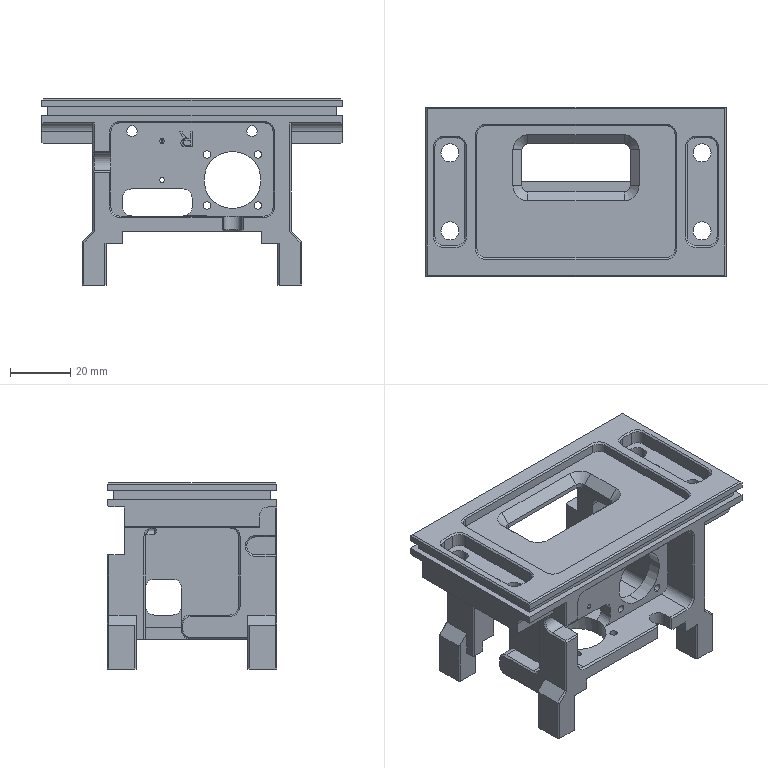NC program | Mastercam | posted with a generic post | part box 100 x 56.5 x 62 mm
Lines 28426 to 30392 of 45570, first 1501 of 1967 lines:
N6980 T16 M6
N6990 G0 G90 G17 G54 X59.6 Y2.263 A0. S5500 M3
N7000 G43 H16 Z20. M8
N7010 Z1.
N7020 G1 Z-28.5 F600.
N7030 X58.469 Y1.131 F1000.
N7040 G3 X58. Y0. I1.131 J-1.131
N7050 G1 Y-31.
N7060 G2 X50. Y-39. I-8. J0.
N7070 G1 X-50.
N7080 G2 X-58. Y-31. I0. J8.
N7090 G1 Y31.
N7100 G2 X-50. Y39. I8. J0.
N7110 G1 X50.
N7120 G2 X58. Y31. I0. J-8.
N7130 G1 Y0.
N7140 Y-.5
N7150 G3 X58.469 Y-1.631 I1.6 J0.
N7160 G1 X59.6 Y-2.763
N7170 Y2.263
N7180 Z-57. F600.
N7190 X58.469 Y1.131 F1000.
N7200 G3 X58. Y0. I1.131 J-1.131
N7210 G1 Y-31.
N7220 G2 X50. Y-39. I-8. J0.
N7230 G1 X-50.
N7240 G2 X-58. Y-31. I0. J8.
N7250 G1 Y31.
N7260 G2 X-50. Y39. I8. J0.
N7270 G1 X50.
N7280 G2 X58. Y31. I0. J-8.
N7290 G1 Y0.
N7300 Y-.5
N7310 G3 X58.469 Y-1.631 I1.6 J0.
N7320 G1 X59.6 Y-2.763
N7330 G0 Z20.
N7340 M5
N7350 G91 G28 Z0. M9
N7360 A0.
N7370 M01
N7380 T6 M6
N7390 G0 G90 G17 G54 X16.314 Y-19.3 A0. S7000 M3
N7400 G43 H6 Z20. M8
N7410 Z1.
N7420 G1 Z-.496 F600.
N7430 X16.738 Y-19.724 F3000.
N7440 G3 X17.162 Y-19.9 I.424 J.424
N7450 G1 X23.9
N7460 Y-13.87
N7470 G3 X23.724 Y-13.445 I-.6 J0.
N7480 G1 X23.3 Y-13.021
N7490 X16.314 Y-19.3
N7500 Z-.992 F600.
N7510 X16.738 Y-19.724 F3000.
N7520 G3 X17.162 Y-19.9 I.424 J.424
N7530 G1 X23.9
N7540 Y-13.87
N7550 G3 X23.724 Y-13.445 I-.6 J0.
N7560 G1 X23.3 Y-13.021
N7570 X16.314 Y-19.3
N7580 Z-1.488 F600.
N7590 X16.738 Y-19.724 F3000.
N7600 G3 X17.162 Y-19.9 I.424 J.424
N7610 G1 X23.9
N7620 Y-13.87
N7630 G3 X23.724 Y-13.445 I-.6 J0.
N7640 G1 X23.3 Y-13.021
N7650 X16.314 Y-19.3
N7660 Z-1.983 F600.
N7670 X16.738 Y-19.724 F3000.
N7680 G3 X17.162 Y-19.9 I.424 J.424
N7690 G1 X23.9
N7700 Y-13.87
N7710 G3 X23.724 Y-13.445 I-.6 J0.
N7720 G1 X23.3 Y-13.021
N7730 X16.314 Y-19.3
N7740 Z-2.479 F600.
N7750 X16.738 Y-19.724 F3000.
N7760 G3 X17.162 Y-19.9 I.424 J.424
N7770 G1 X23.9
N7780 Y-13.87
N7790 G3 X23.724 Y-13.445 I-.6 J0.
N7800 G1 X23.3 Y-13.021
N7810 X16.314 Y-19.3
N7820 Z-2.975 F600.
N7830 X16.738 Y-19.724 F3000.
N7840 G3 X17.162 Y-19.9 I.424 J.424
N7850 G1 X23.9
N7860 Y-13.87
N7870 G3 X23.724 Y-13.445 I-.6 J0.
N7880 G1 X23.3 Y-13.021
N7890 X16.314 Y-19.3
N7900 Z-3.471 F600.
N7910 X16.738 Y-19.724 F3000.
N7920 G3 X17.162 Y-19.9 I.424 J.424
N7930 G1 X23.9
N7940 Y-13.87
N7950 G3 X23.724 Y-13.445 I-.6 J0.
N7960 G1 X23.3 Y-13.021
N7970 X16.314 Y-19.3
N7980 Z-3.967 F600.
N7990 X16.738 Y-19.724 F3000.
N8000 G3 X17.162 Y-19.9 I.424 J.424
N8010 G1 X23.9
N8020 Y-13.87
N8030 G3 X23.724 Y-13.445 I-.6 J0.
N8040 G1 X23.3 Y-13.021
N8050 X16.314 Y-19.3
N8060 Z-4.463 F600.
N8070 X16.738 Y-19.724 F3000.
N8080 G3 X17.162 Y-19.9 I.424 J.424
N8090 G1 X23.9
N8100 Y-13.87
N8110 G3 X23.724 Y-13.445 I-.6 J0.
N8120 G1 X23.3 Y-13.021
N8130 X16.314 Y-19.3
N8140 Z-4.958 F600.
N8150 X16.738 Y-19.724 F3000.
N8160 G3 X17.162 Y-19.9 I.424 J.424
N8170 G1 X23.9
N8180 Y-13.87
N8190 G3 X23.724 Y-13.445 I-.6 J0.
N8200 G1 X23.3 Y-13.021
N8210 X16.314 Y-19.3
N8220 Z-5.454 F600.
N8230 X16.738 Y-19.724 F3000.
N8240 G3 X17.162 Y-19.9 I.424 J.424
N8250 G1 X23.9
N8260 Y-13.87
N8270 G3 X23.724 Y-13.445 I-.6 J0.
N8280 G1 X23.3 Y-13.021
N8290 X16.314 Y-19.3
N8300 Z-5.95 F600.
N8310 X16.738 Y-19.724 F3000.
N8320 G3 X17.162 Y-19.9 I.424 J.424
N8330 G1 X23.9
N8340 Y-13.87
N8350 G3 X23.724 Y-13.445 I-.6 J0.
N8360 G1 X23.3 Y-13.021
N8370 X16.314 Y-19.3
N8380 Z-6.446 F600.
N8390 X16.738 Y-19.724 F3000.
N8400 G3 X17.162 Y-19.9 I.424 J.424
N8410 G1 X23.9
N8420 Y-13.87
N8430 G3 X23.724 Y-13.445 I-.6 J0.
N8440 G1 X23.3 Y-13.021
N8450 X16.314 Y-19.3
N8460 Z-6.942 F600.
N8470 X16.738 Y-19.724 F3000.
N8480 G3 X17.162 Y-19.9 I.424 J.424
N8490 G1 X23.9
N8500 Y-13.87
N8510 G3 X23.724 Y-13.445 I-.6 J0.
N8520 G1 X23.3 Y-13.021
N8530 X16.314 Y-19.3
N8540 Z-7.438 F600.
N8550 X16.738 Y-19.724 F3000.
N8560 G3 X17.162 Y-19.9 I.424 J.424
N8570 G1 X23.9
N8580 Y-13.87
N8590 G3 X23.724 Y-13.445 I-.6 J0.
N8600 G1 X23.3 Y-13.021
N8610 X16.314 Y-19.3
N8620 Z-7.933 F600.
N8630 X16.738 Y-19.724 F3000.
N8640 G3 X17.162 Y-19.9 I.424 J.424
N8650 G1 X23.9
N8660 Y-13.87
N8670 G3 X23.724 Y-13.445 I-.6 J0.
N8680 G1 X23.3 Y-13.021
N8690 X16.314 Y-19.3
N8700 Z-8.429 F600.
N8710 X16.738 Y-19.724 F3000.
N8720 G3 X17.162 Y-19.9 I.424 J.424
N8730 G1 X23.9
N8740 Y-13.87
N8750 G3 X23.724 Y-13.445 I-.6 J0.
N8760 G1 X23.3 Y-13.021
N8770 X16.314 Y-19.3
N8780 Z-8.925 F600.
N8790 X16.738 Y-19.724 F3000.
N8800 G3 X17.162 Y-19.9 I.424 J.424
N8810 G1 X23.9
N8820 Y-13.87
N8830 G3 X23.724 Y-13.445 I-.6 J0.
N8840 G1 X23.3 Y-13.021
N8850 X16.314 Y-19.3
N8860 Z-9.421 F600.
N8870 X16.738 Y-19.724 F3000.
N8880 G3 X17.162 Y-19.9 I.424 J.424
N8890 G1 X23.9
N8900 Y-13.87
N8910 G3 X23.724 Y-13.445 I-.6 J0.
N8920 G1 X23.3 Y-13.021
N8930 X16.314 Y-19.3
N8940 Z-9.917 F600.
N8950 X16.738 Y-19.724 F3000.
N8960 G3 X17.162 Y-19.9 I.424 J.424
N8970 G1 X23.9
N8980 Y-13.87
N8990 G3 X23.724 Y-13.445 I-.6 J0.
N9000 G1 X23.3 Y-13.021
N9010 X16.314 Y-19.3
N9020 Z-10.412 F600.
N9030 X16.738 Y-19.724 F3000.
N9040 G3 X17.162 Y-19.9 I.424 J.424
N9050 G1 X23.9
N9060 Y-13.87
N9070 G3 X23.724 Y-13.445 I-.6 J0.
N9080 G1 X23.3 Y-13.021
N9090 X16.314 Y-19.3
N9100 Z-10.908 F600.
N9110 X16.738 Y-19.724 F3000.
N9120 G3 X17.162 Y-19.9 I.424 J.424
N9130 G1 X23.9
N9140 Y-13.87
N9150 G3 X23.724 Y-13.445 I-.6 J0.
N9160 G1 X23.3 Y-13.021
N9170 X16.314 Y-19.3
N9180 Z-11.404 F600.
N9190 X16.738 Y-19.724 F3000.
N9200 G3 X17.162 Y-19.9 I.424 J.424
N9210 G1 X23.9
N9220 Y-13.87
N9230 G3 X23.724 Y-13.445 I-.6 J0.
N9240 G1 X23.3 Y-13.021
N9250 X16.314 Y-19.3
N9260 Z-11.9 F600.
N9270 X16.738 Y-19.724 F3000.
N9280 G3 X17.162 Y-19.9 I.424 J.424
N9290 G1 X23.9
N9300 Y-13.87
N9310 G3 X23.724 Y-13.445 I-.6 J0.
N9320 G1 X23.3 Y-13.021
N9330 G0 Z20.
N9340 X-23.3
N9350 Z1.
N9360 G1 Z-.496 F600.
N9370 X-23.724 Y-13.445 F3000.
N9380 G3 X-23.9 Y-13.869 I.424 J-.424
N9390 G1 Y-19.9
N9400 X-17.162
N9410 G3 X-16.738 Y-19.724 I0. J.6
N9420 G1 X-16.314 Y-19.3
N9430 X-23.3 Y-13.021
N9440 Z-.992 F600.
N9450 X-23.724 Y-13.445 F3000.
N9460 G3 X-23.9 Y-13.869 I.424 J-.424
N9470 G1 Y-19.9
N9480 X-17.162
N9490 G3 X-16.738 Y-19.724 I0. J.6
N9500 G1 X-16.314 Y-19.3
N9510 X-23.3 Y-13.021
N9520 Z-1.488 F600.
N9530 X-23.724 Y-13.445 F3000.
N9540 G3 X-23.9 Y-13.869 I.424 J-.424
N9550 G1 Y-19.9
N9560 X-17.162
N9570 G3 X-16.738 Y-19.724 I0. J.6
N9580 G1 X-16.314 Y-19.3
N9590 X-23.3 Y-13.021
N9600 Z-1.983 F600.
N9610 X-23.724 Y-13.445 F3000.
N9620 G3 X-23.9 Y-13.869 I.424 J-.424
N9630 G1 Y-19.9
N9640 X-17.162
N9650 G3 X-16.738 Y-19.724 I0. J.6
N9660 G1 X-16.314 Y-19.3
N9670 X-23.3 Y-13.021
N9680 Z-2.479 F600.
N9690 X-23.724 Y-13.445 F3000.
N9700 G3 X-23.9 Y-13.869 I.424 J-.424
N9710 G1 Y-19.9
N9720 X-17.162
N9730 G3 X-16.738 Y-19.724 I0. J.6
N9740 G1 X-16.314 Y-19.3
N9750 X-23.3 Y-13.021
N9760 Z-2.975 F600.
N9770 X-23.724 Y-13.445 F3000.
N9780 G3 X-23.9 Y-13.869 I.424 J-.424
N9790 G1 Y-19.9
N9800 X-17.162
N9810 G3 X-16.738 Y-19.724 I0. J.6
N9820 G1 X-16.314 Y-19.3
N9830 X-23.3 Y-13.021
N9840 Z-3.471 F600.
N9850 X-23.724 Y-13.445 F3000.
N9860 G3 X-23.9 Y-13.869 I.424 J-.424
N9870 G1 Y-19.9
N9880 X-17.162
N9890 G3 X-16.738 Y-19.724 I0. J.6
N9900 G1 X-16.314 Y-19.3
N9910 X-23.3 Y-13.021
N9920 Z-3.967 F600.
N9930 X-23.724 Y-13.445 F3000.
N9940 G3 X-23.9 Y-13.869 I.424 J-.424
N9950 G1 Y-19.9
N9960 X-17.162
N9970 G3 X-16.738 Y-19.724 I0. J.6
N9980 G1 X-16.314 Y-19.3
N9990 X-23.3 Y-13.021
N100 Z-4.463 F600.
N110 X-23.724 Y-13.445 F3000.
N120 G3 X-23.9 Y-13.869 I.424 J-.424
N130 G1 Y-19.9
N140 X-17.162
N150 G3 X-16.738 Y-19.724 I0. J.6
N160 G1 X-16.314 Y-19.3
N170 X-23.3 Y-13.021
N180 Z-4.958 F600.
N190 X-23.724 Y-13.445 F3000.
N200 G3 X-23.9 Y-13.869 I.424 J-.424
N210 G1 Y-19.9
N220 X-17.162
N230 G3 X-16.738 Y-19.724 I0. J.6
N240 G1 X-16.314 Y-19.3
N250 X-23.3 Y-13.021
N260 Z-5.454 F600.
N270 X-23.724 Y-13.445 F3000.
N280 G3 X-23.9 Y-13.869 I.424 J-.424
N290 G1 Y-19.9
N300 X-17.162
N310 G3 X-16.738 Y-19.724 I0. J.6
N320 G1 X-16.314 Y-19.3
N330 X-23.3 Y-13.021
N340 Z-5.95 F600.
N350 X-23.724 Y-13.445 F3000.
N360 G3 X-23.9 Y-13.869 I.424 J-.424
N370 G1 Y-19.9
N380 X-17.162
N390 G3 X-16.738 Y-19.724 I0. J.6
N400 G1 X-16.314 Y-19.3
N410 X-23.3 Y-13.021
N420 Z-6.446 F600.
N430 X-23.724 Y-13.445 F3000.
N440 G3 X-23.9 Y-13.869 I.424 J-.424
N450 G1 Y-19.9
N460 X-17.162
N470 G3 X-16.738 Y-19.724 I0. J.6
N480 G1 X-16.314 Y-19.3
N490 X-23.3 Y-13.021
N500 Z-6.942 F600.
N510 X-23.724 Y-13.445 F3000.
N520 G3 X-23.9 Y-13.869 I.424 J-.424
N530 G1 Y-19.9
N540 X-17.162
N550 G3 X-16.738 Y-19.724 I0. J.6
N560 G1 X-16.314 Y-19.3
N570 X-23.3 Y-13.021
N580 Z-7.438 F600.
N590 X-23.724 Y-13.445 F3000.
N600 G3 X-23.9 Y-13.869 I.424 J-.424
N610 G1 Y-19.9
N620 X-17.162
N630 G3 X-16.738 Y-19.724 I0. J.6
N640 G1 X-16.314 Y-19.3
N650 X-23.3 Y-13.021
N660 Z-7.933 F600.
N670 X-23.724 Y-13.445 F3000.
N680 G3 X-23.9 Y-13.869 I.424 J-.424
N690 G1 Y-19.9
N700 X-17.162
N710 G3 X-16.738 Y-19.724 I0. J.6
N720 G1 X-16.314 Y-19.3
N730 X-23.3 Y-13.021
N740 Z-8.429 F600.
N750 X-23.724 Y-13.445 F3000.
N760 G3 X-23.9 Y-13.869 I.424 J-.424
N770 G1 Y-19.9
N780 X-17.162
N790 G3 X-16.738 Y-19.724 I0. J.6
N800 G1 X-16.314 Y-19.3
N810 X-23.3 Y-13.021
N820 Z-8.925 F600.
N830 X-23.724 Y-13.445 F3000.
N840 G3 X-23.9 Y-13.869 I.424 J-.424
N850 G1 Y-19.9
N860 X-17.162
N870 G3 X-16.738 Y-19.724 I0. J.6
N880 G1 X-16.314 Y-19.3
N890 X-23.3 Y-13.021
N900 Z-9.421 F600.
N910 X-23.724 Y-13.445 F3000.
N920 G3 X-23.9 Y-13.869 I.424 J-.424
N930 G1 Y-19.9
N940 X-17.162
N950 G3 X-16.738 Y-19.724 I0. J.6
N960 G1 X-16.314 Y-19.3
N970 X-23.3 Y-13.021
N980 Z-9.917 F600.
N990 X-23.724 Y-13.445 F3000.
N1000 G3 X-23.9 Y-13.869 I.424 J-.424
N1010 G1 Y-19.9
N1020 X-17.162
N1030 G3 X-16.738 Y-19.724 I0. J.6
N1040 G1 X-16.314 Y-19.3
N1050 X-23.3 Y-13.021
N1060 Z-10.412 F600.
N1070 X-23.724 Y-13.445 F3000.
N1080 G3 X-23.9 Y-13.869 I.424 J-.424
N1090 G1 Y-19.9
N1100 X-17.162
N1110 G3 X-16.738 Y-19.724 I0. J.6
N1120 G1 X-16.314 Y-19.3
N1130 X-23.3 Y-13.021
N1140 Z-10.908 F600.
N1150 X-23.724 Y-13.445 F3000.
N1160 G3 X-23.9 Y-13.869 I.424 J-.424
N1170 G1 Y-19.9
N1180 X-17.162
N1190 G3 X-16.738 Y-19.724 I0. J.6
N1200 G1 X-16.314 Y-19.3
N1210 X-23.3 Y-13.021
N1220 Z-11.404 F600.
N1230 X-23.724 Y-13.445 F3000.
N1240 G3 X-23.9 Y-13.869 I.424 J-.424
N1250 G1 Y-19.9
N1260 X-17.162
N1270 G3 X-16.738 Y-19.724 I0. J.6
N1280 G1 X-16.314 Y-19.3
N1290 X-23.3 Y-13.021
N1300 Z-11.9 F600.
N1310 X-23.724 Y-13.445 F3000.
N1320 G3 X-23.9 Y-13.869 I.424 J-.424
N1330 G1 Y-19.9
N1340 X-17.162
N1350 G3 X-16.738 Y-19.724 I0. J.6
N1360 G1 X-16.314 Y-19.3
N1370 G0 Z20.
N1380 X-16.603 Y4.3
N1390 Z1.
N1400 G1 Z-.496 F600.
N1410 X-17.027 Y4.724 F3000.
N1420 G3 X-17.451 Y4.9 I-.424 J-.424
N1430 G1 X-23.9
N1440 Y-1.142
N1450 G3 X-23.724 Y-1.567 I.6 J0.
N1460 G1 X-23.3 Y-1.991
N1470 X-16.603 Y4.3
N1480 Z-.992 F600.
N1490 X-17.027 Y4.724 F3000.
N1500 G3 X-17.451 Y4.9 I-.424 J-.424
N1510 G1 X-23.9
N1520 Y-1.142
N1530 G3 X-23.724 Y-1.567 I.6 J0.
N1540 G1 X-23.3 Y-1.991
N1550 X-16.603 Y4.3
N1560 Z-1.488 F600.
N1570 X-17.027 Y4.724 F3000.
N1580 G3 X-17.451 Y4.9 I-.424 J-.424
N1590 G1 X-23.9
N1600 Y-1.142
N1610 G3 X-23.724 Y-1.567 I.6 J0.
N1620 G1 X-23.3 Y-1.991
N1630 X-16.603 Y4.3
N1640 Z-1.983 F600.
N1650 X-17.027 Y4.724 F3000.
N1660 G3 X-17.451 Y4.9 I-.424 J-.424
N1670 G1 X-23.9
N1680 Y-1.142
N1690 G3 X-23.724 Y-1.567 I.6 J0.
N1700 G1 X-23.3 Y-1.991
N1710 X-16.603 Y4.3
N1720 Z-2.479 F600.
N1730 X-17.027 Y4.724 F3000.
N1740 G3 X-17.451 Y4.9 I-.424 J-.424
N1750 G1 X-23.9
N1760 Y-1.142
N1770 G3 X-23.724 Y-1.567 I.6 J0.
N1780 G1 X-23.3 Y-1.991
N1790 X-16.603 Y4.3
N1800 Z-2.975 F600.
N1810 X-17.027 Y4.724 F3000.
N1820 G3 X-17.451 Y4.9 I-.424 J-.424
N1830 G1 X-23.9
N1840 Y-1.142
N1850 G3 X-23.724 Y-1.567 I.6 J0.
N1860 G1 X-23.3 Y-1.991
N1870 X-16.603 Y4.3
N1880 Z-3.471 F600.
N1890 X-17.027 Y4.724 F3000.
N1900 G3 X-17.451 Y4.9 I-.424 J-.424
N1910 G1 X-23.9
N1920 Y-1.142
N1930 G3 X-23.724 Y-1.567 I.6 J0.
N1940 G1 X-23.3 Y-1.991
N1950 X-16.603 Y4.3
N1960 Z-3.967 F600.
N1970 X-17.027 Y4.724 F3000.
N1980 G3 X-17.451 Y4.9 I-.424 J-.424
N1990 G1 X-23.9
N2000 Y-1.142
N2010 G3 X-23.724 Y-1.567 I.6 J0.
N2020 G1 X-23.3 Y-1.991
N2030 X-16.603 Y4.3
N2040 Z-4.463 F600.
N2050 X-17.027 Y4.724 F3000.
N2060 G3 X-17.451 Y4.9 I-.424 J-.424
N2070 G1 X-23.9
N2080 Y-1.142
N2090 G3 X-23.724 Y-1.567 I.6 J0.
N2100 G1 X-23.3 Y-1.991
N2110 X-16.603 Y4.3
N2120 Z-4.958 F600.
N2130 X-17.027 Y4.724 F3000.
N2140 G3 X-17.451 Y4.9 I-.424 J-.424
N2150 G1 X-23.9
N2160 Y-1.142
N2170 G3 X-23.724 Y-1.567 I.6 J0.
N2180 G1 X-23.3 Y-1.991
N2190 X-16.603 Y4.3
N2200 Z-5.454 F600.
N2210 X-17.027 Y4.724 F3000.
N2220 G3 X-17.451 Y4.9 I-.424 J-.424
N2230 G1 X-23.9
N2240 Y-1.142
N2250 G3 X-23.724 Y-1.567 I.6 J0.
N2260 G1 X-23.3 Y-1.991
N2270 X-16.603 Y4.3
N2280 Z-5.95 F600.
N2290 X-17.027 Y4.724 F3000.
N2300 G3 X-17.451 Y4.9 I-.424 J-.424
N2310 G1 X-23.9
N2320 Y-1.142
N2330 G3 X-23.724 Y-1.567 I.6 J0.
N2340 G1 X-23.3 Y-1.991
N2350 X-16.603 Y4.3
N2360 Z-6.446 F600.
N2370 X-17.027 Y4.724 F3000.
N2380 G3 X-17.451 Y4.9 I-.424 J-.424
N2390 G1 X-23.9
N2400 Y-1.142
N2410 G3 X-23.724 Y-1.567 I.6 J0.
N2420 G1 X-23.3 Y-1.991
N2430 X-16.603 Y4.3
N2440 Z-6.942 F600.
N2450 X-17.027 Y4.724 F3000.
N2460 G3 X-17.451 Y4.9 I-.424 J-.424
N2470 G1 X-23.9
N2480 Y-1.142
N2490 G3 X-23.724 Y-1.567 I.6 J0.
N2500 G1 X-23.3 Y-1.991
N2510 X-16.603 Y4.3
N2520 Z-7.438 F600.
N2530 X-17.027 Y4.724 F3000.
N2540 G3 X-17.451 Y4.9 I-.424 J-.424
N2550 G1 X-23.9
N2560 Y-1.142
N2570 G3 X-23.724 Y-1.567 I.6 J0.
N2580 G1 X-23.3 Y-1.991
N2590 X-16.603 Y4.3
N2600 Z-7.933 F600.
N2610 X-17.027 Y4.724 F3000.
N2620 G3 X-17.451 Y4.9 I-.424 J-.424
N2630 G1 X-23.9
N2640 Y-1.142
N2650 G3 X-23.724 Y-1.567 I.6 J0.
N2660 G1 X-23.3 Y-1.991
N2670 X-16.603 Y4.3
N2680 Z-8.429 F600.
N2690 X-17.027 Y4.724 F3000.
N2700 G3 X-17.451 Y4.9 I-.424 J-.424
N2710 G1 X-23.9
N2720 Y-1.142
N2730 G3 X-23.724 Y-1.567 I.6 J0.
N2740 G1 X-23.3 Y-1.991
N2750 X-16.603 Y4.3
N2760 Z-8.925 F600.
N2770 X-17.027 Y4.724 F3000.
N2780 G3 X-17.451 Y4.9 I-.424 J-.424
N2790 G1 X-23.9
N2800 Y-1.142
N2810 G3 X-23.724 Y-1.567 I.6 J0.
N2820 G1 X-23.3 Y-1.991
N2830 X-16.603 Y4.3
N2840 Z-9.421 F600.
N2850 X-17.027 Y4.724 F3000.
N2860 G3 X-17.451 Y4.9 I-.424 J-.424
N2870 G1 X-23.9
N2880 Y-1.142
N2890 G3 X-23.724 Y-1.567 I.6 J0.
N2900 G1 X-23.3 Y-1.991
N2910 X-16.603 Y4.3
N2920 Z-9.917 F600.
N2930 X-17.027 Y4.724 F3000.
N2940 G3 X-17.451 Y4.9 I-.424 J-.424
N2950 G1 X-23.9
N2960 Y-1.142
N2970 G3 X-23.724 Y-1.567 I.6 J0.
N2980 G1 X-23.3 Y-1.991
N2990 X-16.603 Y4.3
N3000 Z-10.412 F600.
N3010 X-17.027 Y4.724 F3000.
N3020 G3 X-17.451 Y4.9 I-.424 J-.424
N3030 G1 X-23.9
N3040 Y-1.142
N3050 G3 X-23.724 Y-1.567 I.6 J0.
N3060 G1 X-23.3 Y-1.991
N3070 X-16.603 Y4.3
N3080 Z-10.908 F600.
N3090 X-17.027 Y4.724 F3000.
N3100 G3 X-17.451 Y4.9 I-.424 J-.424
N3110 G1 X-23.9
N3120 Y-1.142
N3130 G3 X-23.724 Y-1.567 I.6 J0.
N3140 G1 X-23.3 Y-1.991
N3150 X-16.603 Y4.3
N3160 Z-11.404 F600.
N3170 X-17.027 Y4.724 F3000.
N3180 G3 X-17.451 Y4.9 I-.424 J-.424
N3190 G1 X-23.9
N3200 Y-1.142
N3210 G3 X-23.724 Y-1.567 I.6 J0.
N3220 G1 X-23.3 Y-1.991
N3230 X-16.603 Y4.3
N3240 Z-11.9 F600.
N3250 X-17.027 Y4.724 F3000.
N3260 G3 X-17.451 Y4.9 I-.424 J-.424
N3270 G1 X-23.9
N3280 Y-1.142
N3290 G3 X-23.724 Y-1.567 I.6 J0.
N3300 G1 X-23.3 Y-1.991
N3310 G0 Z20.
N3320 X23.3 Y-1.99
N3330 Z1.
N3340 G1 Z-.496 F600.
N3350 X23.724 Y-1.566 F3000.
N3360 G3 X23.9 Y-1.142 I-.424 J.424
N3370 G1 Y4.9
N3380 X17.451
N3390 G3 X17.027 Y4.724 I0. J-.6
N3400 G1 X16.603 Y4.3
N3410 X23.3 Y-1.99
N3420 Z-.992 F600.
N3430 X23.724 Y-1.566 F3000.
N3440 G3 X23.9 Y-1.142 I-.424 J.424
N3450 G1 Y4.9
N3460 X17.451
N3470 G3 X17.027 Y4.724 I0. J-.6
N3480 G1 X16.603 Y4.3
N3490 X23.3 Y-1.99
N3500 Z-1.488 F600.
N3510 X23.724 Y-1.566 F3000.
N3520 G3 X23.9 Y-1.142 I-.424 J.424
N3530 G1 Y4.9
N3540 X17.451
N3550 G3 X17.027 Y4.724 I0. J-.6
N3560 G1 X16.603 Y4.3
N3570 X23.3 Y-1.99
N3580 Z-1.983 F600.
N3590 X23.724 Y-1.566 F3000.
N3600 G3 X23.9 Y-1.142 I-.424 J.424
N3610 G1 Y4.9
N3620 X17.451
N3630 G3 X17.027 Y4.724 I0. J-.6
N3640 G1 X16.603 Y4.3
N3650 X23.3 Y-1.99
N3660 Z-2.479 F600.
N3670 X23.724 Y-1.566 F3000.
N3680 G3 X23.9 Y-1.142 I-.424 J.424
N3690 G1 Y4.9
N3700 X17.451
N3710 G3 X17.027 Y4.724 I0. J-.6
N3720 G1 X16.603 Y4.3
N3730 X23.3 Y-1.99
N3740 Z-2.975 F600.
N3750 X23.724 Y-1.566 F3000.
N3760 G3 X23.9 Y-1.142 I-.424 J.424
N3770 G1 Y4.9
N3780 X17.451
N3790 G3 X17.027 Y4.724 I0. J-.6
N3800 G1 X16.603 Y4.3
N3810 X23.3 Y-1.99
N3820 Z-3.471 F600.
N3830 X23.724 Y-1.566 F3000.
N3840 G3 X23.9 Y-1.142 I-.424 J.424
N3850 G1 Y4.9
N3860 X17.451
N3870 G3 X17.027 Y4.724 I0. J-.6
N3880 G1 X16.603 Y4.3
N3890 X23.3 Y-1.99
N3900 Z-3.967 F600.
N3910 X23.724 Y-1.566 F3000.
N3920 G3 X23.9 Y-1.142 I-.424 J.424
N3930 G1 Y4.9
N3940 X17.451
N3950 G3 X17.027 Y4.724 I0. J-.6
N3960 G1 X16.603 Y4.3
N3970 X23.3 Y-1.99
N3980 Z-4.463 F600.
N3990 X23.724 Y-1.566 F3000.
N4000 G3 X23.9 Y-1.142 I-.424 J.424
N4010 G1 Y4.9
N4020 X17.451
N4030 G3 X17.027 Y4.724 I0. J-.6
N4040 G1 X16.603 Y4.3
N4050 X23.3 Y-1.99
N4060 Z-4.958 F600.
N4070 X23.724 Y-1.566 F3000.
N4080 G3 X23.9 Y-1.142 I-.424 J.424
N4090 G1 Y4.9
N4100 X17.451
N4110 G3 X17.027 Y4.724 I0. J-.6
N4120 G1 X16.603 Y4.3
N4130 X23.3 Y-1.99
N4140 Z-5.454 F600.
N4150 X23.724 Y-1.566 F3000.
N4160 G3 X23.9 Y-1.142 I-.424 J.424
N4170 G1 Y4.9
N4180 X17.451
N4190 G3 X17.027 Y4.724 I0. J-.6
N4200 G1 X16.603 Y4.3
N4210 X23.3 Y-1.99
N4220 Z-5.95 F600.
N4230 X23.724 Y-1.566 F3000.
N4240 G3 X23.9 Y-1.142 I-.424 J.424
N4250 G1 Y4.9
N4260 X17.451
N4270 G3 X17.027 Y4.724 I0. J-.6
N4280 G1 X16.603 Y4.3
N4290 X23.3 Y-1.99
N4300 Z-6.446 F600.
N4310 X23.724 Y-1.566 F3000.
N4320 G3 X23.9 Y-1.142 I-.424 J.424
N4330 G1 Y4.9
N4340 X17.451
N4350 G3 X17.027 Y4.724 I0. J-.6
N4360 G1 X16.603 Y4.3
N4370 X23.3 Y-1.99
N4380 Z-6.942 F600.
N4390 X23.724 Y-1.566 F3000.
N4400 G3 X23.9 Y-1.142 I-.424 J.424
N4410 G1 Y4.9
N4420 X17.451
N4430 G3 X17.027 Y4.724 I0. J-.6
N4440 G1 X16.603 Y4.3
N4450 X23.3 Y-1.99
N4460 Z-7.438 F600.
N4470 X23.724 Y-1.566 F3000.
N4480 G3 X23.9 Y-1.142 I-.424 J.424
N4490 G1 Y4.9
N4500 X17.451
N4510 G3 X17.027 Y4.724 I0. J-.6
N4520 G1 X16.603 Y4.3
N4530 X23.3 Y-1.99
N4540 Z-7.933 F600.
N4550 X23.724 Y-1.566 F3000.
N4560 G3 X23.9 Y-1.142 I-.424 J.424
N4570 G1 Y4.9
N4580 X17.451
N4590 G3 X17.027 Y4.724 I0. J-.6
N4600 G1 X16.603 Y4.3
N4610 X23.3 Y-1.99
N4620 Z-8.429 F600.
N4630 X23.724 Y-1.566 F3000.
N4640 G3 X23.9 Y-1.142 I-.424 J.424
N4650 G1 Y4.9
N4660 X17.451
N4670 G3 X17.027 Y4.724 I0. J-.6
N4680 G1 X16.603 Y4.3
N4690 X23.3 Y-1.99
N4700 Z-8.925 F600.
N4710 X23.724 Y-1.566 F3000.
N4720 G3 X23.9 Y-1.142 I-.424 J.424
N4730 G1 Y4.9
N4740 X17.451
N4750 G3 X17.027 Y4.724 I0. J-.6
N4760 G1 X16.603 Y4.3
N4770 X23.3 Y-1.99
N4780 Z-9.421 F600.
N4790 X23.724 Y-1.566 F3000.
N4800 G3 X23.9 Y-1.142 I-.424 J.424
N4810 G1 Y4.9
N4820 X17.451
N4830 G3 X17.027 Y4.724 I0. J-.6
N4840 G1 X16.603 Y4.3
N4850 X23.3 Y-1.99
N4860 Z-9.917 F600.
N4870 X23.724 Y-1.566 F3000.
N4880 G3 X23.9 Y-1.142 I-.424 J.424
N4890 G1 Y4.9
N4900 X17.451
N4910 G3 X17.027 Y4.724 I0. J-.6
N4920 G1 X16.603 Y4.3
N4930 X23.3 Y-1.99
N4940 Z-10.412 F600.
N4950 X23.724 Y-1.566 F3000.
N4960 G3 X23.9 Y-1.142 I-.424 J.424
N4970 G1 Y4.9
N4980 X17.451
N4990 G3 X17.027 Y4.724 I0. J-.6
N5000 G1 X16.603 Y4.3
N5010 X23.3 Y-1.99
N5020 Z-10.908 F600.
N5030 X23.724 Y-1.566 F3000.
N5040 G3 X23.9 Y-1.142 I-.424 J.424
N5050 G1 Y4.9
N5060 X17.451
N5070 G3 X17.027 Y4.724 I0. J-.6
N5080 G1 X16.603 Y4.3
N5090 X23.3 Y-1.99
N5100 Z-11.404 F600.
N5110 X23.724 Y-1.566 F3000.
N5120 G3 X23.9 Y-1.142 I-.424 J.424
N5130 G1 Y4.9
N5140 X17.451
N5150 G3 X17.027 Y4.724 I0. J-.6
N5160 G1 X16.603 Y4.3
N5170 X23.3 Y-1.99
N5180 Z-11.9 F600.
N5190 X23.724 Y-1.566 F3000.
N5200 G3 X23.9 Y-1.142 I-.424 J.424
N5210 G1 Y4.9
N5220 X17.451
N5230 G3 X17.027 Y4.724 I0. J-.6
N5240 G1 X16.603 Y4.3
N5250 G0 Z20.
N5260 X-5.901 Y4.4
N5270 Z1.
N5280 G1 Z-5.99 F600.
N5290 X-6.326 Y4.824 F1000.
N5300 G3 X-6.75 Y5. I-.424 J-.424
N5310 G1 X-24.
N5320 Y-7.
N5330 Y-13.
N5340 Y-20.
N5350 X24.
N5360 Y5.
N5370 X16.5
N5380 X10.5
N5390 X-6.75
N5400 X-7.25
N5410 G3 X-7.674 Y4.824 I0. J-.6
N5420 G1 X-8.099 Y4.4
N5430 X-5.901
N5440 Z-11.98 F600.
N5450 X-6.326 Y4.824 F1000.
N5460 G3 X-6.75 Y5. I-.424 J-.424
N5470 G1 X-24.
N5480 Y-7.
N5490 Y-13.
N5500 Y-20.
N5510 X24.
N5520 Y5.
N5530 X16.5
N5540 X10.5
N5550 X-6.75
N5560 X-7.25
N5570 G3 X-7.674 Y4.824 I0. J-.6
N5580 G1 X-8.099 Y4.4
N5590 X-5.901 F500.
N5600 Z-12. F600.
N5610 X-6.326 Y4.824 F500.
N5620 G3 X-6.75 Y5. I-.424 J-.424
N5630 G1 X-24.
N5640 Y-7.
N5650 Y-13.
N5660 Y-20.
N5670 X24.
N5680 Y5.
N5690 X16.5
N5700 X10.5
N5710 X-6.75
N5720 X-7.25
N5730 G3 X-7.674 Y4.824 I0. J-.6
N5740 G1 X-8.099 Y4.4
N5750 G0 Z20.
N5760 X-1.856 Y-6.821
N5770 Z-11.
N5780 G1 Z-11.7 F600.
N5790 G3 X-7.556 Y-12.521 Z-11.775 I0. J-5.7 F1000.
N5800 X-1.856 Y-18.221 Z-11.85 I5.7 J0.
N5810 X3.844 Y-12.521 Z-11.925 I0. J5.7
N5820 X-1.856 Y-6.821 Z-12. I-5.7 J0.
N5830 G1 X-12.179
N5840 Y-8.179
N5850 X0.
N5860 X12.179
N5870 Y-6.821
N5880 X-1.856
N5890 G2 X-2.46 Y-6.335 I0. J.619
N5900 G1 X-3.108 Y-3.399
N5910 G3 X-3.712 Y-2.914 I-.604 J-.133
N5920 G1 X-16.086
N5930 Y-12.086
N5940 X0.
N5950 X16.086
N5960 Y-2.914
N5970 X-3.712
N5980 G2 X-4.317 Y-2.428 I0. J.619
N5990 G1 X-4.965 Y.508
N6000 G3 X-5.569 Y.993 I-.604 J-.134
N6010 G1 X-19.993
N6020 Y-15.993
N6030 X0.
N6040 X19.993
N6050 Y.993
N6060 X-5.569
N6070 G2 X-6.173 Y1.479 I0. J.619
N6080 G1 X-6.821 Y4.415
N6090 G3 X-7.425 Y4.9 I-.604 J-.134
N6100 G1 X-23.46
N6110 X-23.887 Y4.889
N6120 X-23.9 Y4.721
N6130 Y-19.721
N6140 X-23.887 Y-19.889
N6150 X-23.46 Y-19.9
N6160 X0.
N6170 X23.46
N6180 X23.887 Y-19.889
N6190 X23.9 Y-19.721
N6200 Y4.721
N6210 X23.887 Y4.889
N6220 X23.46 Y4.9
N6230 X-7.425
N6240 G0 Z20.
N6250 X13.5 Y-1.1
N6260 Z-11.
N6270 G1 Z-12. F600.
N6280 X12.749 Y-1.199 Z-12.021 F1500.
N6290 X12.05 Y-1.489 Z-12.042
N6300 X11.449 Y-1.949 Z-12.063
N6310 X10.989 Y-2.55 Z-12.083
N6320 X10.699 Y-3.249 Z-12.104
N6330 X10.6 Y-4. Z-12.125
N6340 X10.699 Y-4.751 Z-12.146
N6350 X10.989 Y-5.45 Z-12.167
N6360 X11.449 Y-6.051 Z-12.188
N6370 X12.05 Y-6.511 Z-12.208
N6380 X12.749 Y-6.801 Z-12.229
N6390 X13.5 Y-6.9 Z-12.25
N6400 X14.251 Y-6.801 Z-12.271
N6410 X14.95 Y-6.511 Z-12.292
N6420 X15.551 Y-6.051 Z-12.313
N6430 X16.011 Y-5.45 Z-12.333
N6440 X16.301 Y-4.751 Z-12.354
N6450 X16.4 Y-4. Z-12.375
N6460 X16.301 Y-3.249 Z-12.396
N6470 X16.011 Y-2.55 Z-12.417
N6480 X15.551 Y-1.949 Z-12.438
N6490 X14.95 Y-1.489 Z-12.458
N6500 X14.251 Y-1.199 Z-12.479
N6510 X13.5 Y-1.1 Z-12.5
N6520 X12.749 Y-1.199 Z-12.521
N6530 X12.05 Y-1.489 Z-12.542
N6540 X11.449 Y-1.949 Z-12.563
N6550 X10.989 Y-2.55 Z-12.583
N6560 X10.699 Y-3.249 Z-12.604
N6570 X10.6 Y-4. Z-12.625
N6580 X10.699 Y-4.751 Z-12.646
N6590 X10.989 Y-5.45 Z-12.667
N6600 X11.449 Y-6.051 Z-12.688
N6610 X12.05 Y-6.511 Z-12.708
N6620 X12.749 Y-6.801 Z-12.729
N6630 X13.5 Y-6.9 Z-12.75
N6640 X14.251 Y-6.801 Z-12.771
N6650 X14.95 Y-6.511 Z-12.792
N6660 X15.551 Y-6.051 Z-12.813
N6670 X16.011 Y-5.45 Z-12.833
N6680 X16.301 Y-4.751 Z-12.854
N6690 X16.4 Y-4. Z-12.875
N6700 X16.301 Y-3.249 Z-12.896
N6710 X16.011 Y-2.55 Z-12.917
N6720 X15.551 Y-1.949 Z-12.938
N6730 X14.95 Y-1.489 Z-12.958
N6740 X14.251 Y-1.199 Z-12.979
N6750 X13.5 Y-1.1 Z-13.
N6760 X12.749 Y-1.199 Z-13.021
N6770 X12.05 Y-1.489 Z-13.042
N6780 X11.449 Y-1.949 Z-13.063
N6790 X10.989 Y-2.55 Z-13.083
N6800 X10.699 Y-3.249 Z-13.104
N6810 X10.6 Y-4. Z-13.125
N6820 X10.699 Y-4.751 Z-13.146
N6830 X10.989 Y-5.45 Z-13.167
N6840 X11.449 Y-6.051 Z-13.188
N6850 X12.05 Y-6.511 Z-13.208
N6860 X12.749 Y-6.801 Z-13.229
N6870 X13.5 Y-6.9 Z-13.25
N6880 X14.251 Y-6.801 Z-13.271
N6890 X14.95 Y-6.511 Z-13.292
N6900 X15.551 Y-6.051 Z-13.313
N6910 X16.011 Y-5.45 Z-13.333
N6920 X16.301 Y-4.751 Z-13.354
N6930 X16.4 Y-4. Z-13.375
N6940 X16.301 Y-3.249 Z-13.396
N6950 X16.011 Y-2.55 Z-13.417
N6960 X15.551 Y-1.949 Z-13.438
N6970 X14.95 Y-1.489 Z-13.458
N6980 X14.251 Y-1.199 Z-13.479
N6990 X13.5 Y-1.1 Z-13.5
N7000 X12.749 Y-1.199 Z-13.521
N7010 X12.05 Y-1.489 Z-13.542
N7020 X11.449 Y-1.949 Z-13.563
N7030 X10.989 Y-2.55 Z-13.583
N7040 X10.699 Y-3.249 Z-13.604
N7050 X10.6 Y-4. Z-13.625
N7060 X10.699 Y-4.751 Z-13.646
N7070 X10.989 Y-5.45 Z-13.667
N7080 X11.449 Y-6.051 Z-13.688
N7090 X12.05 Y-6.511 Z-13.708
N7100 X12.749 Y-6.801 Z-13.729
N7110 X13.5 Y-6.9 Z-13.75
N7120 X14.251 Y-6.801 Z-13.771
N7130 X14.95 Y-6.511 Z-13.792
N7140 X15.551 Y-6.051 Z-13.813
N7150 X16.011 Y-5.45 Z-13.833
N7160 X16.301 Y-4.751 Z-13.854
N7170 X16.4 Y-4. Z-13.875
N7180 X16.301 Y-3.249 Z-13.896
N7190 X16.011 Y-2.55 Z-13.917
N7200 X15.551 Y-1.949 Z-13.938
N7210 X14.95 Y-1.489 Z-13.958
N7220 X14.251 Y-1.199 Z-13.979
N7230 X13.5 Y-1.1 Z-14.
N7240 X12.749 Y-1.199 Z-14.021
N7250 X12.05 Y-1.489 Z-14.042
N7260 X11.449 Y-1.949 Z-14.063
N7270 X10.989 Y-2.55 Z-14.083
N7280 X10.699 Y-3.249 Z-14.104
N7290 X10.6 Y-4. Z-14.125
N7300 X10.699 Y-4.751 Z-14.146
N7310 X10.989 Y-5.45 Z-14.167
N7320 X11.449 Y-6.051 Z-14.188
N7330 X12.05 Y-6.511 Z-14.208
N7340 X12.749 Y-6.801 Z-14.229
N7350 X13.5 Y-6.9 Z-14.25
N7360 X14.251 Y-6.801 Z-14.271
N7370 X14.95 Y-6.511 Z-14.292
N7380 X15.551 Y-6.051 Z-14.313
N7390 X16.011 Y-5.45 Z-14.333
N7400 X16.301 Y-4.751 Z-14.354
N7410 X16.4 Y-4. Z-14.375
N7420 X16.301 Y-3.249 Z-14.396
N7430 X16.011 Y-2.55 Z-14.417
N7440 X15.551 Y-1.949 Z-14.438
N7450 X14.95 Y-1.489 Z-14.458
N7460 X14.251 Y-1.199 Z-14.479
N7470 X13.5 Y-1.1 Z-14.5
N7480 X12.749 Y-1.199 Z-14.521
N7490 X12.05 Y-1.489 Z-14.542
N7500 X11.449 Y-1.949 Z-14.563
N7510 X10.989 Y-2.55 Z-14.583
N7520 X10.699 Y-3.249 Z-14.604
N7530 X10.6 Y-4. Z-14.625
N7540 X10.699 Y-4.751 Z-14.646
N7550 X10.989 Y-5.45 Z-14.667
N7560 X11.449 Y-6.051 Z-14.688
N7570 X12.05 Y-6.511 Z-14.708
N7580 X12.749 Y-6.801 Z-14.729
N7590 X13.5 Y-6.9 Z-14.75
N7600 X14.251 Y-6.801 Z-14.771
N7610 X14.95 Y-6.511 Z-14.792
N7620 X15.551 Y-6.051 Z-14.813
N7630 X16.011 Y-5.45 Z-14.833
N7640 X16.301 Y-4.751 Z-14.854
N7650 X16.4 Y-4. Z-14.875
N7660 X16.301 Y-3.249 Z-14.896
N7670 X16.011 Y-2.55 Z-14.917
N7680 X15.551 Y-1.949 Z-14.938
N7690 X14.95 Y-1.489 Z-14.958
N7700 X14.251 Y-1.199 Z-14.979
N7710 X13.5 Y-1.1 Z-15.
N7720 X12.749 Y-1.199 Z-15.021
N7730 X12.05 Y-1.489 Z-15.042
N7740 X11.449 Y-1.949 Z-15.063
N7750 X10.989 Y-2.55 Z-15.083
N7760 X10.699 Y-3.249 Z-15.104
N7770 X10.6 Y-4. Z-15.125
N7780 X10.699 Y-4.751 Z-15.146
N7790 X10.989 Y-5.45 Z-15.167
N7800 X11.449 Y-6.051 Z-15.188
N7810 X12.05 Y-6.511 Z-15.208
N7820 X12.749 Y-6.801 Z-15.229
N7830 X13.5 Y-6.9 Z-15.25
N7840 X14.251 Y-6.801 Z-15.271
N7850 X14.95 Y-6.511 Z-15.292
N7860 X15.551 Y-6.051 Z-15.313
N7870 X16.011 Y-5.45 Z-15.333
N7880 X16.301 Y-4.751 Z-15.354
N7890 X16.4 Y-4. Z-15.375
N7900 X16.301 Y-3.249 Z-15.396
N7910 X16.011 Y-2.55 Z-15.417
N7920 X15.551 Y-1.949 Z-15.438
N7930 X14.95 Y-1.489 Z-15.458
N7940 X14.251 Y-1.199 Z-15.479
N7950 X13.5 Y-1.1 Z-15.5
N7960 X12.749 Y-1.199 Z-15.521
N7970 X12.05 Y-1.489 Z-15.542
N7980 X11.449 Y-1.949 Z-15.563
N7990 X10.989 Y-2.55 Z-15.583
N8000 X10.699 Y-3.249 Z-15.604
N8010 X10.6 Y-4. Z-15.625
N8020 X10.699 Y-4.751 Z-15.646
N8030 X10.989 Y-5.45 Z-15.667
N8040 X11.449 Y-6.051 Z-15.688
N8050 X12.05 Y-6.511 Z-15.708
N8060 X12.749 Y-6.801 Z-15.729
N8070 X13.5 Y-6.9 Z-15.75
N8080 X14.251 Y-6.801 Z-15.771
N8090 X14.95 Y-6.511 Z-15.792
N8100 X15.551 Y-6.051 Z-15.813
N8110 X16.011 Y-5.45 Z-15.833
N8120 X16.301 Y-4.751 Z-15.854
N8130 X16.4 Y-4. Z-15.875
N8140 X16.301 Y-3.249 Z-15.896
N8150 X16.011 Y-2.55 Z-15.917
N8160 X15.551 Y-1.949 Z-15.938
N8170 X14.95 Y-1.489 Z-15.958
N8180 X14.251 Y-1.199 Z-15.979
N8190 X13.5 Y-1.1 Z-16.
N8200 X12.749 Y-1.199 Z-16.021
N8210 X12.05 Y-1.489 Z-16.042
N8220 X11.449 Y-1.949 Z-16.063
N8230 X10.989 Y-2.55 Z-16.083
N8240 X10.699 Y-3.249 Z-16.104
N8250 X10.6 Y-4. Z-16.125
N8260 X10.699 Y-4.751 Z-16.146
N8270 X10.989 Y-5.45 Z-16.167
N8280 X11.449 Y-6.051 Z-16.188
N8290 X12.05 Y-6.511 Z-16.208
N8300 X12.749 Y-6.801 Z-16.229
N8310 X13.5 Y-6.9 Z-16.25
N8320 X14.251 Y-6.801 Z-16.271
N8330 X14.95 Y-6.511 Z-16.292
N8340 X15.551 Y-6.051 Z-16.313
N8350 X16.011 Y-5.45 Z-16.333
N8360 X16.301 Y-4.751 Z-16.354
N8370 X16.4 Y-4. Z-16.375
N8380 X16.301 Y-3.249 Z-16.396
N8390 X16.011 Y-2.55 Z-16.417
N8400 X15.551 Y-1.949 Z-16.438
N8410 X14.95 Y-1.489 Z-16.458
N8420 X14.251 Y-1.199 Z-16.479
N8430 X13.5 Y-1.1 Z-16.5
N8440 X12.749 Y-1.199 Z-16.521
N8450 X12.05 Y-1.489 Z-16.542
N8460 X11.449 Y-1.949 Z-16.563
N8470 X10.989 Y-2.55 Z-16.583
N8480 X10.699 Y-3.249 Z-16.604
N8490 X10.6 Y-4. Z-16.625
N8500 X10.699 Y-4.751 Z-16.646
N8510 X10.989 Y-5.45 Z-16.667
N8520 X11.449 Y-6.051 Z-16.688
N8530 X12.05 Y-6.511 Z-16.708
N8540 X12.749 Y-6.801 Z-16.729
N8550 X13.5 Y-6.9 Z-16.75
N8560 X14.251 Y-6.801 Z-16.771
N8570 X14.95 Y-6.511 Z-16.792
N8580 X15.551 Y-6.051 Z-16.813
N8590 X16.011 Y-5.45 Z-16.833
N8600 X16.301 Y-4.751 Z-16.854
N8610 X16.4 Y-4. Z-16.875
N8620 X16.301 Y-3.249 Z-16.896
N8630 X16.011 Y-2.55 Z-16.917
N8640 X15.551 Y-1.949 Z-16.938
N8650 X14.95 Y-1.489 Z-16.958
N8660 X14.251 Y-1.199 Z-16.979
N8670 X13.5 Y-1.1 Z-17.
N8680 G3 X10.6 Y-4. I0. J-2.9
N8690 X13.5 Y-6.9 I2.9 J0.
N8700 X16.4 Y-4. I0. J2.9
N8710 X13.5 Y-1.1 I-2.9 J0.
N8720 X13.002 Y-1.143 I0. J-2.9
N8730 G0 Z20.
N8740 X13.5 Y2.4
N8750 Z-11.
N8760 G1 Z-12. F600.
N8770 X12.389 Y2.303 Z-12.014 F1500.
N8780 X11.311 Y2.014 Z-12.028
N8790 X10.3 Y1.543 Z-12.042
N8800 X9.386 Y.903 Z-12.056
N8810 X8.597 Y.114 Z-12.069
N8820 X7.957 Y-.8 Z-12.083
N8830 X7.486 Y-1.811 Z-12.097
N8840 X7.197 Y-2.889 Z-12.111
N8850 X7.1 Y-4. Z-12.125
N8860 X7.197 Y-5.111 Z-12.139
N8870 X7.486 Y-6.189 Z-12.153
N8880 X7.957 Y-7.2 Z-12.167
N8890 X8.597 Y-8.114 Z-12.181
N8900 X9.386 Y-8.903 Z-12.194
N8910 X10.3 Y-9.543 Z-12.208
N8920 X11.311 Y-10.014 Z-12.222
N8930 X12.389 Y-10.303 Z-12.236
N8940 X13.5 Y-10.4 Z-12.25
N8950 X14.611 Y-10.303 Z-12.264
N8960 X15.689 Y-10.014 Z-12.278
N8970 X16.7 Y-9.543 Z-12.292
N8980 X17.614 Y-8.903 Z-12.306
N8990 X18.403 Y-8.114 Z-12.319
N9000 X19.043 Y-7.2 Z-12.333
N9010 X19.514 Y-6.189 Z-12.347
N9020 X19.803 Y-5.111 Z-12.361
N9030 X19.9 Y-4. Z-12.375
N9040 X19.803 Y-2.889 Z-12.389
N9050 X19.514 Y-1.811 Z-12.403
N9060 X19.043 Y-.8 Z-12.417
N9070 X18.403 Y.114 Z-12.431
N9080 X17.614 Y.903 Z-12.444
N9090 X16.7 Y1.543 Z-12.458
N9100 X15.689 Y2.014 Z-12.472
N9110 X14.611 Y2.303 Z-12.486
N9120 X13.5 Y2.4 Z-12.5
N9130 X12.389 Y2.303 Z-12.514
N9140 X11.311 Y2.014 Z-12.528
N9150 X10.3 Y1.543 Z-12.542
N9160 X9.386 Y.903 Z-12.556
N9170 X8.597 Y.114 Z-12.569
N9180 X7.957 Y-.8 Z-12.583
N9190 X7.486 Y-1.811 Z-12.597
N9200 X7.197 Y-2.889 Z-12.611
N9210 X7.1 Y-4. Z-12.625
N9220 X7.197 Y-5.111 Z-12.639
N9230 X7.486 Y-6.189 Z-12.653
N9240 X7.957 Y-7.2 Z-12.667
N9250 X8.597 Y-8.114 Z-12.681
N9260 X9.386 Y-8.903 Z-12.694
N9270 X10.3 Y-9.543 Z-12.708
N9280 X11.311 Y-10.014 Z-12.722
N9290 X12.389 Y-10.303 Z-12.736
N9300 X13.5 Y-10.4 Z-12.75
N9310 X14.611 Y-10.303 Z-12.764
N9320 X15.689 Y-10.014 Z-12.778
N9330 X16.7 Y-9.543 Z-12.792
N9340 X17.614 Y-8.903 Z-12.806
N9350 X18.403 Y-8.114 Z-12.819
N9360 X19.043 Y-7.2 Z-12.833
N9370 X19.514 Y-6.189 Z-12.847
N9380 X19.803 Y-5.111 Z-12.861
N9390 X19.9 Y-4. Z-12.875
N9400 X19.803 Y-2.889 Z-12.889
N9410 X19.514 Y-1.811 Z-12.903
N9420 X19.043 Y-.8 Z-12.917
N9430 X18.403 Y.114 Z-12.931
N9440 X17.614 Y.903 Z-12.944
N9450 X16.7 Y1.543 Z-12.958
N9460 X15.689 Y2.014 Z-12.972
N9470 X14.611 Y2.303 Z-12.986
N9480 X13.5 Y2.4 Z-13.
N9490 X12.389 Y2.303 Z-13.014
N9500 X11.311 Y2.014 Z-13.028
N9510 X10.3 Y1.543 Z-13.042
N9520 X9.386 Y.903 Z-13.056
N9530 X8.597 Y.114 Z-13.069
N9540 X7.957 Y-.8 Z-13.083
N9550 X7.486 Y-1.811 Z-13.097
N9560 X7.197 Y-2.889 Z-13.111
N9570 X7.1 Y-4. Z-13.125
N9580 X7.197 Y-5.111 Z-13.139
N9590 X7.486 Y-6.189 Z-13.153
N9600 X7.957 Y-7.2 Z-13.167
N9610 X8.597 Y-8.114 Z-13.181
N9620 X9.386 Y-8.903 Z-13.194
N9630 X10.3 Y-9.543 Z-13.208
N9640 X11.311 Y-10.014 Z-13.222
N9650 X12.389 Y-10.303 Z-13.236
N9660 X13.5 Y-10.4 Z-13.25
N9670 X14.611 Y-10.303 Z-13.264
N9680 X15.689 Y-10.014 Z-13.278
N9690 X16.7 Y-9.543 Z-13.292
N9700 X17.614 Y-8.903 Z-13.306
N9710 X18.403 Y-8.114 Z-13.319
N9720 X19.043 Y-7.2 Z-13.333
N9730 X19.514 Y-6.189 Z-13.347
N9740 X19.803 Y-5.111 Z-13.361
N9750 X19.9 Y-4. Z-13.375
N9760 X19.803 Y-2.889 Z-13.389
N9770 X19.514 Y-1.811 Z-13.403
N9780 X19.043 Y-.8 Z-13.417
N9790 X18.403 Y.114 Z-13.431
N9800 X17.614 Y.903 Z-13.444
N9810 X16.7 Y1.543 Z-13.458
N9820 X15.689 Y2.014 Z-13.472
N9830 X14.611 Y2.303 Z-13.486
N9840 X13.5 Y2.4 Z-13.5
N9850 X12.389 Y2.303 Z-13.514
N9860 X11.311 Y2.014 Z-13.528
N9870 X10.3 Y1.543 Z-13.542
N9880 X9.386 Y.903 Z-13.556
N9890 X8.597 Y.114 Z-13.569
N9900 X7.957 Y-.8 Z-13.583
N9910 X7.486 Y-1.811 Z-13.597
N9920 X7.197 Y-2.889 Z-13.611
N9930 X7.1 Y-4. Z-13.625
N9940 X7.197 Y-5.111 Z-13.639
N9950 X7.486 Y-6.189 Z-13.653
N9960 X7.957 Y-7.2 Z-13.667
N9970 X8.597 Y-8.114 Z-13.681
N9980 X9.386 Y-8.903 Z-13.694
N9990 X10.3 Y-9.543 Z-13.708
N100 X11.311 Y-10.014 Z-13.722
N110 X12.389 Y-10.303 Z-13.736
N120 X13.5 Y-10.4 Z-13.75
N130 X14.611 Y-10.303 Z-13.764
N140 X15.689 Y-10.014 Z-13.778
N150 X16.7 Y-9.543 Z-13.792
N160 X17.614 Y-8.903 Z-13.806
N170 X18.403 Y-8.114 Z-13.819
N180 X19.043 Y-7.2 Z-13.833
N190 X19.514 Y-6.189 Z-13.847
N200 X19.803 Y-5.111 Z-13.861
N210 X19.9 Y-4. Z-13.875
N220 X19.803 Y-2.889 Z-13.889
N230 X19.514 Y-1.811 Z-13.903
N240 X19.043 Y-.8 Z-13.917
N250 X18.403 Y.114 Z-13.931
N260 X17.614 Y.903 Z-13.944
N270 X16.7 Y1.543 Z-13.958
N280 X15.689 Y2.014 Z-13.972
N290 X14.611 Y2.303 Z-13.986
N300 X13.5 Y2.4 Z-14.
N310 X12.389 Y2.303 Z-14.014
N320 X11.311 Y2.014 Z-14.028
N330 X10.3 Y1.543 Z-14.042
N340 X9.386 Y.903 Z-14.056
N350 X8.597 Y.114 Z-14.069
N360 X7.957 Y-.8 Z-14.083
N370 X7.486 Y-1.811 Z-14.097
N380 X7.197 Y-2.889 Z-14.111
N390 X7.1 Y-4. Z-14.125
N400 X7.197 Y-5.111 Z-14.139
N410 X7.486 Y-6.189 Z-14.153
N420 X7.957 Y-7.2 Z-14.167
N430 X8.597 Y-8.114 Z-14.181
N440 X9.386 Y-8.903 Z-14.194
N450 X10.3 Y-9.543 Z-14.208
N460 X11.311 Y-10.014 Z-14.222
N470 X12.389 Y-10.303 Z-14.236
N480 X13.5 Y-10.4 Z-14.25
N490 X14.611 Y-10.303 Z-14.264
N500 X15.689 Y-10.014 Z-14.278
N510 X16.7 Y-9.543 Z-14.292
N520 X17.614 Y-8.903 Z-14.306
N530 X18.403 Y-8.114 Z-14.319
N540 X19.043 Y-7.2 Z-14.333
N550 X19.514 Y-6.189 Z-14.347
N560 X19.803 Y-5.111 Z-14.361
N570 X19.9 Y-4. Z-14.375
N580 X19.803 Y-2.889 Z-14.389
N590 X19.514 Y-1.811 Z-14.403
N600 X19.043 Y-.8 Z-14.417
N610 X18.403 Y.114 Z-14.431
N620 X17.614 Y.903 Z-14.444
N630 X16.7 Y1.543 Z-14.458
N640 X15.689 Y2.014 Z-14.472
N650 X14.611 Y2.303 Z-14.486
N660 X13.5 Y2.4 Z-14.5
N670 X12.389 Y2.303 Z-14.514
N680 X11.311 Y2.014 Z-14.528
N690 X10.3 Y1.543 Z-14.542
N700 X9.386 Y.903 Z-14.556
N710 X8.597 Y.114 Z-14.569
N720 X7.957 Y-.8 Z-14.583
N730 X7.486 Y-1.811 Z-14.597
N740 X7.197 Y-2.889 Z-14.611
N750 X7.1 Y-4. Z-14.625
N760 X7.197 Y-5.111 Z-14.639
N770 X7.486 Y-6.189 Z-14.653
N780 X7.957 Y-7.2 Z-14.667
N790 X8.597 Y-8.114 Z-14.681
N800 X9.386 Y-8.903 Z-14.694
N810 X10.3 Y-9.543 Z-14.708
N820 X11.311 Y-10.014 Z-14.722
N830 X12.389 Y-10.303 Z-14.736
N840 X13.5 Y-10.4 Z-14.75
N850 X14.611 Y-10.303 Z-14.764
N860 X15.689 Y-10.014 Z-14.778
N870 X16.7 Y-9.543 Z-14.792
N880 X17.614 Y-8.903 Z-14.806
N890 X18.403 Y-8.114 Z-14.819
N900 X19.043 Y-7.2 Z-14.833
N910 X19.514 Y-6.189 Z-14.847
N920 X19.803 Y-5.111 Z-14.861
N930 X19.9 Y-4. Z-14.875
N940 X19.803 Y-2.889 Z-14.889
N950 X19.514 Y-1.811 Z-14.903
N960 X19.043 Y-.8 Z-14.917
N970 X18.403 Y.114 Z-14.931
N980 X17.614 Y.903 Z-14.944
N990 X16.7 Y1.543 Z-14.958
N1000 X15.689 Y2.014 Z-14.972
N1010 X14.611 Y2.303 Z-14.986
N1020 X13.5 Y2.4 Z-15.
N1030 X12.389 Y2.303 Z-15.014
N1040 X11.311 Y2.014 Z-15.028
N1050 X10.3 Y1.543 Z-15.042
N1060 X9.386 Y.903 Z-15.056
N1070 X8.597 Y.114 Z-15.069
N1080 X7.957 Y-.8 Z-15.083
N1090 X7.486 Y-1.811 Z-15.097
N1100 X7.197 Y-2.889 Z-15.111
N1110 X7.1 Y-4. Z-15.125
N1120 X7.197 Y-5.111 Z-15.139
N1130 X7.486 Y-6.189 Z-15.153
N1140 X7.957 Y-7.2 Z-15.167
N1150 X8.597 Y-8.114 Z-15.181
N1160 X9.386 Y-8.903 Z-15.194
N1170 X10.3 Y-9.543 Z-15.208
N1180 X11.311 Y-10.014 Z-15.222
N1190 X12.389 Y-10.303 Z-15.236
N1200 X13.5 Y-10.4 Z-15.25
N1210 X14.611 Y-10.303 Z-15.264
N1220 X15.689 Y-10.014 Z-15.278
N1230 X16.7 Y-9.543 Z-15.292
N1240 X17.614 Y-8.903 Z-15.306
N1250 X18.403 Y-8.114 Z-15.319
N1260 X19.043 Y-7.2 Z-15.333
N1270 X19.514 Y-6.189 Z-15.347
N1280 X19.803 Y-5.111 Z-15.361
N1290 X19.9 Y-4. Z-15.375
N1300 X19.803 Y-2.889 Z-15.389
N1310 X19.514 Y-1.811 Z-15.403
N1320 X19.043 Y-.8 Z-15.417
N1330 X18.403 Y.114 Z-15.431
N1340 X17.614 Y.903 Z-15.444
N1350 X16.7 Y1.543 Z-15.458
N1360 X15.689 Y2.014 Z-15.472
N1370 X14.611 Y2.303 Z-15.486
N1380 X13.5 Y2.4 Z-15.5
N1390 X12.389 Y2.303 Z-15.514
N1400 X11.311 Y2.014 Z-15.528
N1410 X10.3 Y1.543 Z-15.542
N1420 X9.386 Y.903 Z-15.556
N1430 X8.597 Y.114 Z-15.569
N1440 X7.957 Y-.8 Z-15.583
N1450 X7.486 Y-1.811 Z-15.597
N1460 X7.197 Y-2.889 Z-15.611
N1470 X7.1 Y-4. Z-15.625
N1480 X7.197 Y-5.111 Z-15.639
N1490 X7.486 Y-6.189 Z-15.653
N1500 X7.957 Y-7.2 Z-15.667
N1510 X8.597 Y-8.114 Z-15.681
N1520 X9.386 Y-8.903 Z-15.694
N1530 X10.3 Y-9.543 Z-15.708
N1540 X11.311 Y-10.014 Z-15.722
N1550 X12.389 Y-10.303 Z-15.736
N1560 X13.5 Y-10.4 Z-15.75
N1570 X14.611 Y-10.303 Z-15.764
N1580 X15.689 Y-10.014 Z-15.778
N1590 X16.7 Y-9.543 Z-15.792
N1600 X17.614 Y-8.903 Z-15.806
N1610 X18.403 Y-8.114 Z-15.819
N1620 X19.043 Y-7.2 Z-15.833
N1630 X19.514 Y-6.189 Z-15.847
N1640 X19.803 Y-5.111 Z-15.861
N1650 X19.9 Y-4. Z-15.875
N1660 X19.803 Y-2.889 Z-15.889
N1670 X19.514 Y-1.811 Z-15.903
N1680 X19.043 Y-.8 Z-15.917
N1690 X18.403 Y.114 Z-15.931
N1700 X17.614 Y.903 Z-15.944
N1710 X16.7 Y1.543 Z-15.958
N1720 X15.689 Y2.014 Z-15.972
N1730 X14.611 Y2.303 Z-15.986
N1740 X13.5 Y2.4 Z-16.
N1750 X12.389 Y2.303 Z-16.014
N1760 X11.311 Y2.014 Z-16.028
N1770 X10.3 Y1.543 Z-16.042
N1780 X9.386 Y.903 Z-16.056
N1790 X8.597 Y.114 Z-16.069
N1800 X7.957 Y-.8 Z-16.083
N1810 X7.486 Y-1.811 Z-16.097
N1820 X7.197 Y-2.889 Z-16.111
N1830 X7.1 Y-4. Z-16.125
N1840 X7.197 Y-5.111 Z-16.139
N1850 X7.486 Y-6.189 Z-16.153
N1860 X7.957 Y-7.2 Z-16.167
N1870 X8.597 Y-8.114 Z-16.181
N1880 X9.386 Y-8.903 Z-16.194
N1890 X10.3 Y-9.543 Z-16.208
N1900 X11.311 Y-10.014 Z-16.222
N1910 X12.389 Y-10.303 Z-16.236
N1920 X13.5 Y-10.4 Z-16.25
N1930 X14.611 Y-10.303 Z-16.264
N1940 X15.689 Y-10.014 Z-16.278
N1950 X16.7 Y-9.543 Z-16.292
N1960 X17.614 Y-8.903 Z-16.306
N1970 X18.403 Y-8.114 Z-16.319
N1980 X19.043 Y-7.2 Z-16.333
N1990 X19.514 Y-6.189 Z-16.347
N2000 X19.803 Y-5.111 Z-16.361
N2010 X19.9 Y-4. Z-16.375
N2020 X19.803 Y-2.889 Z-16.389
N2030 X19.514 Y-1.811 Z-16.403
N2040 X19.043 Y-.8 Z-16.417
N2050 X18.403 Y.114 Z-16.431
N2060 X17.614 Y.903 Z-16.444
N2070 X16.7 Y1.543 Z-16.458
N2080 X15.689 Y2.014 Z-16.472
N2090 X14.611 Y2.303 Z-16.486
N2100 X13.5 Y2.4 Z-16.5
N2110 X12.389 Y2.303 Z-16.514
N2120 X11.311 Y2.014 Z-16.528
N2130 X10.3 Y1.543 Z-16.542
N2140 X9.386 Y.903 Z-16.556
N2150 X8.597 Y.114 Z-16.569
N2160 X7.957 Y-.8 Z-16.583
N2170 X7.486 Y-1.811 Z-16.597
N2180 X7.197 Y-2.889 Z-16.611